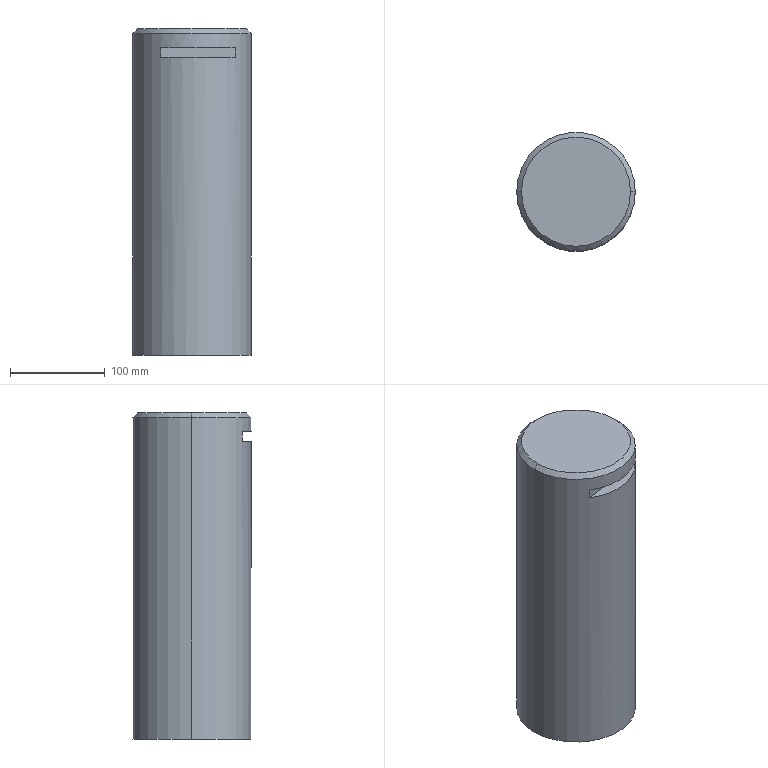Part | SolidWorks | features ICE 2, Chamfer 1, Extrusion 1, MoveFace 1 | 1 solid | 9 faces | box 125 x 125 x 344 mm | volume 4209039 mm3 | plane 5 | cone 2 | cylinder 2 | commonest cylinder face diameters 125 x2
STEP:
#1=CARTESIAN_POINT('',(5146.911,2238.406,-1.881));
#2=VERTEX_POINT('',#1);
#3=CARTESIAN_POINT('',(5031.911,2238.406,-1.881));
#4=VERTEX_POINT('',#3);
#5=CARTESIAN_POINT('',(5089.411,2238.406,-1.881));
#6=DIRECTION('',(0.,0.,1.));
#7=DIRECTION('',(1.,0.,0.));
#8=AXIS2_PLACEMENT_3D('',#5,#6,#7);
#9=CIRCLE('',#8,57.5);
#10=EDGE_CURVE('',#2,#4,#9,.T.);
#11=ORIENTED_EDGE('',*,*,#10,.F.);
#12=CARTESIAN_POINT('',(5151.911,2238.406,-6.881));
#13=VERTEX_POINT('',#12);
#14=CARTESIAN_POINT('',(5146.911,2238.406,-1.881));
#15=DIRECTION('',(0.7071,0.,-0.7071));
#16=VECTOR('',#15,1000.);
#17=LINE('',#14,#16);
#18=EDGE_CURVE('',#2,#13,#17,.T.);
#19=ORIENTED_EDGE('',*,*,#18,.T.);
#20=CARTESIAN_POINT('',(5026.911,2238.406,-6.881));
#21=VERTEX_POINT('',#20);
#22=CARTESIAN_POINT('',(5089.411,2238.406,-6.881));
#23=DIRECTION('',(0.,0.,-1.));
#24=DIRECTION('',(1.,0.,0.));
#25=AXIS2_PLACEMENT_3D('',#22,#23,#24);
#26=CIRCLE('',#25,62.5);
#27=EDGE_CURVE('',#21,#13,#26,.T.);
#28=ORIENTED_EDGE('',*,*,#27,.F.);
#29=CARTESIAN_POINT('',(5031.911,2238.406,-1.881));
#30=DIRECTION('',(-0.7071,0.,-0.7071));
#31=VECTOR('',#30,1000.);
#32=LINE('',#29,#31);
#33=EDGE_CURVE('',#4,#21,#32,.T.);
#34=ORIENTED_EDGE('',*,*,#33,.F.);
#35=EDGE_LOOP('',(#11,#19,#28,#34));
#36=FACE_OUTER_BOUND('',#35,.T.);
#37=CARTESIAN_POINT('',(5089.411,2238.406,-1.881));
#38=DIRECTION('',(0.,0.,-1.));
#39=DIRECTION('',(-1.,0.,0.));
#40=AXIS2_PLACEMENT_3D('',#37,#38,#39);
#41=CONICAL_SURFACE('',#40,57.5,0.7854);
#42=ADVANCED_FACE('',(#36),#41,.T.);
#43=CARTESIAN_POINT('',(5026.911,2238.406,-345.881));
#44=VERTEX_POINT('',#43);
#45=CARTESIAN_POINT('',(5151.911,2238.406,-345.881));
#46=VERTEX_POINT('',#45);
#47=CARTESIAN_POINT('',(5089.411,2238.406,-345.881));
#48=DIRECTION('',(0.,0.,-1.));
#49=DIRECTION('',(1.,0.,0.));
#50=AXIS2_PLACEMENT_3D('',#47,#48,#49);
#51=CIRCLE('',#50,62.5);
#52=EDGE_CURVE('',#44,#46,#51,.T.);
#53=ORIENTED_EDGE('',*,*,#52,.F.);
#54=CARTESIAN_POINT('',(5026.911,2238.406,-522.657));
#55=DIRECTION('',(0.,0.,1.));
#56=VECTOR('',#55,1000.);
#57=LINE('',#54,#56);
#58=EDGE_CURVE('',#44,#21,#57,.T.);
#59=ORIENTED_EDGE('',*,*,#58,.T.);
#60=ORIENTED_EDGE('',*,*,#27,.T.);
#61=CARTESIAN_POINT('',(5151.911,2238.406,-522.657));
#62=DIRECTION('',(0.,0.,1.));
#63=VECTOR('',#62,1000.);
#64=LINE('',#61,#63);
#65=EDGE_CURVE('',#46,#13,#64,.T.);
#66=ORIENTED_EDGE('',*,*,#65,.F.);
#67=EDGE_LOOP('',(#53,#59,#60,#66));
#68=FACE_OUTER_BOUND('',#67,.T.);
#69=CARTESIAN_POINT('',(5089.411,2238.406,-522.657));
#70=DIRECTION('',(0.,0.,1.));
#71=DIRECTION('',(1.,0.,0.));
#72=AXIS2_PLACEMENT_3D('',#69,#70,#71);
#73=CYLINDRICAL_SURFACE('',#72,62.5);
#74=ADVANCED_FACE('',(#68),#73,.T.);
#75=CARTESIAN_POINT('',(5056.406,2185.331,-31.881));
#76=VERTEX_POINT('',#75);
#77=CARTESIAN_POINT('',(5135.037,2195.692,-31.881));
#78=VERTEX_POINT('',#77);
#79=CARTESIAN_POINT('',(5089.411,2238.406,-31.881));
#80=DIRECTION('',(0.,0.,1.));
#81=DIRECTION('',(1.,0.,0.));
#82=AXIS2_PLACEMENT_3D('',#79,#80,#81);
#83=CIRCLE('',#82,62.5);
#84=EDGE_CURVE('',#76,#78,#83,.T.);
#85=ORIENTED_EDGE('',*,*,#84,.T.);
#86=CARTESIAN_POINT('',(-196.746,1493.143,-31.881));
#87=DIRECTION('',(-0.9914,-0.1306,0.));
#88=VECTOR('',#87,1000.);
#89=LINE('',#86,#88);
#90=EDGE_CURVE('',#78,#76,#89,.T.);
#91=ORIENTED_EDGE('',*,*,#90,.T.);
#92=EDGE_LOOP('',(#85,#91));
#93=FACE_OUTER_BOUND('',#92,.T.);
#94=CARTESIAN_POINT('',(5089.411,2238.406,-31.881));
#95=DIRECTION('',(0.,0.,1.));
#96=DIRECTION('',(1.,0.,0.));
#97=AXIS2_PLACEMENT_3D('',#94,#95,#96);
#98=PLANE('',#97);
#99=ADVANCED_FACE('',(#93),#98,.T.);
#100=ORIENTED_EDGE('',*,*,#58,.F.);
#101=CARTESIAN_POINT('',(5089.411,2238.406,-345.881));
#102=DIRECTION('',(0.,0.,-1.));
#103=DIRECTION('',(1.,0.,0.));
#104=AXIS2_PLACEMENT_3D('',#101,#102,#103);
#105=CIRCLE('',#104,62.5);
#106=EDGE_CURVE('',#46,#44,#105,.T.);
#107=ORIENTED_EDGE('',*,*,#106,.F.);
#108=ORIENTED_EDGE('',*,*,#65,.T.);
#109=CARTESIAN_POINT('',(5089.411,2238.406,-6.881));
#110=DIRECTION('',(0.,0.,-1.));
#111=DIRECTION('',(1.,0.,0.));
#112=AXIS2_PLACEMENT_3D('',#109,#110,#111);
#113=CIRCLE('',#112,62.5);
#114=EDGE_CURVE('',#13,#21,#113,.T.);
#115=ORIENTED_EDGE('',*,*,#114,.T.);
#116=EDGE_LOOP('',(#100,#107,#108,#115));
#117=FACE_OUTER_BOUND('',#116,.T.);
#118=ORIENTED_EDGE('',*,*,#84,.F.);
#119=CARTESIAN_POINT('',(5056.406,2185.331,-21.881));
#120=VERTEX_POINT('',#119);
#121=CARTESIAN_POINT('',(5056.406,2185.331,10.));
#122=DIRECTION('',(0.,0.,-1.));
#123=VECTOR('',#122,1000.);
#124=LINE('',#121,#123);
#125=EDGE_CURVE('',#120,#76,#124,.T.);
#126=ORIENTED_EDGE('',*,*,#125,.F.);
#127=CARTESIAN_POINT('',(5135.037,2195.692,-21.881));
#128=VERTEX_POINT('',#127);
#129=CARTESIAN_POINT('',(5089.411,2238.406,-21.881));
#130=DIRECTION('',(0.,0.,1.));
#131=DIRECTION('',(1.,0.,0.));
#132=AXIS2_PLACEMENT_3D('',#129,#130,#131);
#133=CIRCLE('',#132,62.5);
#134=EDGE_CURVE('',#120,#128,#133,.T.);
#135=ORIENTED_EDGE('',*,*,#134,.T.);
#136=CARTESIAN_POINT('',(5135.037,2195.692,10.));
#137=DIRECTION('',(0.,0.,-1.));
#138=VECTOR('',#137,1000.);
#139=LINE('',#136,#138);
#140=EDGE_CURVE('',#128,#78,#139,.T.);
#141=ORIENTED_EDGE('',*,*,#140,.T.);
#142=EDGE_LOOP('',(#118,#126,#135,#141));
#143=FACE_BOUND('',#142,.T.);
#144=CARTESIAN_POINT('',(5089.411,2238.406,-522.657));
#145=DIRECTION('',(0.,0.,1.));
#146=DIRECTION('',(1.,0.,0.));
#147=AXIS2_PLACEMENT_3D('',#144,#145,#146);
#148=CYLINDRICAL_SURFACE('',#147,62.5);
#149=ADVANCED_FACE('',(#117,#143),#148,.T.);
#150=ORIENTED_EDGE('',*,*,#106,.T.);
#151=ORIENTED_EDGE('',*,*,#52,.T.);
#152=EDGE_LOOP('',(#150,#151));
#153=FACE_OUTER_BOUND('',#152,.T.);
#154=CARTESIAN_POINT('',(5360.292,2632.168,-345.881));
#155=DIRECTION('',(0.,0.,1.));
#156=DIRECTION('',(-0.9914,-0.1306,0.));
#157=AXIS2_PLACEMENT_3D('',#154,#155,#156);
#158=PLANE('',#157);
#159=ADVANCED_FACE('',(#153),#158,.F.);
#160=ORIENTED_EDGE('',*,*,#90,.F.);
#161=ORIENTED_EDGE('',*,*,#140,.F.);
#162=CARTESIAN_POINT('',(-196.746,1493.143,-21.881));
#163=DIRECTION('',(-0.9914,-0.1306,0.));
#164=VECTOR('',#163,1000.);
#165=LINE('',#162,#164);
#166=EDGE_CURVE('',#128,#120,#165,.T.);
#167=ORIENTED_EDGE('',*,*,#166,.T.);
#168=ORIENTED_EDGE('',*,*,#125,.T.);
#169=EDGE_LOOP('',(#160,#161,#167,#168));
#170=FACE_OUTER_BOUND('',#169,.T.);
#171=CARTESIAN_POINT('',(-196.746,1493.143,10.));
#172=DIRECTION('',(0.1306,-0.9914,0.));
#173=DIRECTION('',(0.9914,0.1306,0.));
#174=AXIS2_PLACEMENT_3D('',#171,#172,#173);
#175=PLANE('',#174);
#176=ADVANCED_FACE('',(#170),#175,.T.);
#177=CARTESIAN_POINT('',(5089.411,2238.406,-1.881));
#178=DIRECTION('',(0.,0.,1.));
#179=DIRECTION('',(1.,0.,0.));
#180=AXIS2_PLACEMENT_3D('',#177,#178,#179);
#181=CIRCLE('',#180,57.5);
#182=EDGE_CURVE('',#4,#2,#181,.T.);
#183=ORIENTED_EDGE('',*,*,#182,.T.);
#184=ORIENTED_EDGE('',*,*,#10,.T.);
#185=EDGE_LOOP('',(#183,#184));
#186=FACE_OUTER_BOUND('',#185,.T.);
#187=CARTESIAN_POINT('',(5089.411,2238.406,-1.881));
#188=DIRECTION('',(0.,0.,1.));
#189=DIRECTION('',(1.,0.,0.));
#190=AXIS2_PLACEMENT_3D('',#187,#188,#189);
#191=PLANE('',#190);
#192=ADVANCED_FACE('',(#186),#191,.T.);
#193=ORIENTED_EDGE('',*,*,#166,.F.);
#194=ORIENTED_EDGE('',*,*,#134,.F.);
#195=EDGE_LOOP('',(#193,#194));
#196=FACE_OUTER_BOUND('',#195,.T.);
#197=CARTESIAN_POINT('',(5089.411,2238.406,-21.881));
#198=DIRECTION('',(0.,0.,1.));
#199=DIRECTION('',(1.,0.,0.));
#200=AXIS2_PLACEMENT_3D('',#197,#198,#199);
#201=PLANE('',#200);
#202=ADVANCED_FACE('',(#196),#201,.F.);
#203=ORIENTED_EDGE('',*,*,#18,.F.);
#204=ORIENTED_EDGE('',*,*,#182,.F.);
#205=ORIENTED_EDGE('',*,*,#33,.T.);
#206=ORIENTED_EDGE('',*,*,#114,.F.);
#207=EDGE_LOOP('',(#203,#204,#205,#206));
#208=FACE_OUTER_BOUND('',#207,.T.);
#209=CARTESIAN_POINT('',(5089.411,2238.406,-1.881));
#210=DIRECTION('',(0.,0.,-1.));
#211=DIRECTION('',(-1.,0.,0.));
#212=AXIS2_PLACEMENT_3D('',#209,#210,#211);
#213=CONICAL_SURFACE('',#212,57.5,0.7854);
#214=ADVANCED_FACE('',(#208),#213,.T.);
#215=CLOSED_SHELL('',(#42,#74,#99,#149,#159,#176,#192,#202,#214));
#216=MANIFOLD_SOLID_BREP('',#215);
#217=CARTESIAN_POINT('',(0.,0.,0.));
#218=DIRECTION('',(0.,0.,1.));
#219=DIRECTION('',(1.,0.,0.));
#220=AXIS2_PLACEMENT_3D('',#217,#218,#219);
#221=(LENGTH_UNIT()NAMED_UNIT(*)SI_UNIT(.MILLI.,.METRE.));
#222=UNCERTAINTY_MEASURE_WITH_UNIT(LENGTH_MEASURE(0.00001),#221,'','');
#223=(NAMED_UNIT(*)PLANE_ANGLE_UNIT()SI_UNIT($,.RADIAN.));
#224=(NAMED_UNIT(*)SI_UNIT($,.STERADIAN.)SOLID_ANGLE_UNIT());
#225=(GEOMETRIC_REPRESENTATION_CONTEXT(3)GLOBAL_UNCERTAINTY_ASSIGNED_CONTEXT((#222))GLOBAL_UNIT_ASSIGNED_CONTEXT((#221,#223,#224))REPRESENTATION_CONTEXT('',''));
#226=ADVANCED_BREP_SHAPE_REPRESENTATION('',(#216,#220),#225);